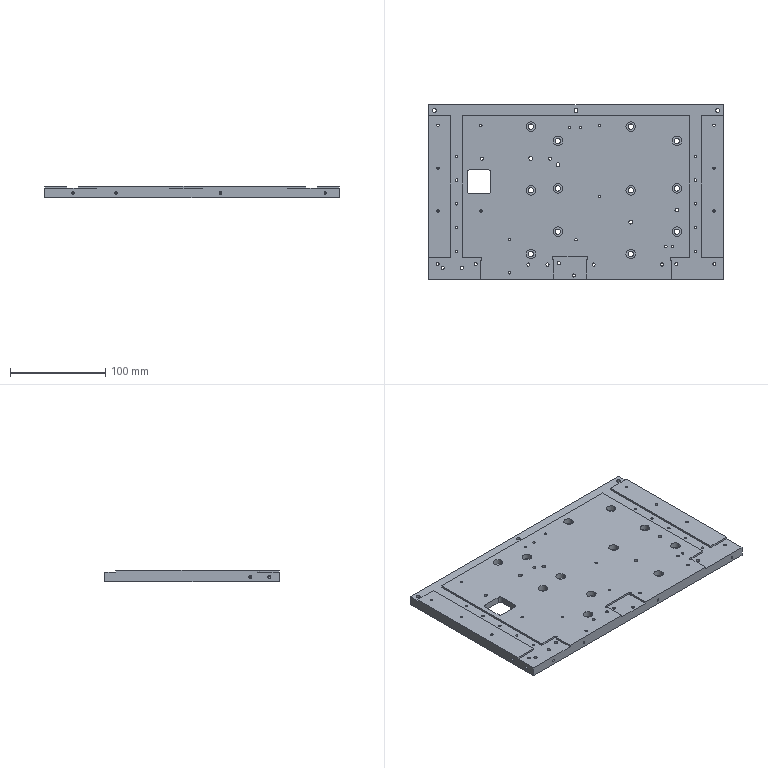Part | NX | features BREP 1 | 1 solid | 274 faces | box 310 x 183.5 x 12 mm | volume 522912 mm3 | cylinder 190 | plane 68 | cone 16 | commonest cylinder face diameters 2.5 x62 3.3 x36 5.5 x24 6 x24 10 x24 4 x8